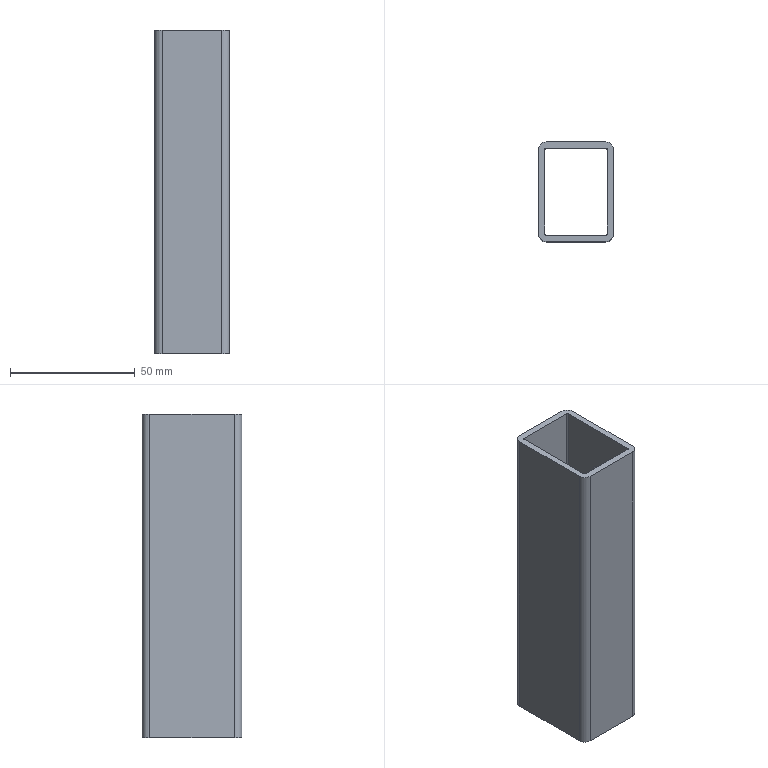Part | SolidWorks | features BaseBody 1 | 1 solid | 22 faces | box 30 x 40 x 130 mm | volume 41175 mm3 | cylinder 12 | plane 10 | commonest cylinder face diameters 1 x4 5 x4 6 x4
STEP:
#1=CARTESIAN_POINT('',(12.5,0.,47.5));
#2=VERTEX_POINT('',#1);
#3=CARTESIAN_POINT('',(15.,0.,47.5));
#4=VERTEX_POINT('',#3);
#5=CARTESIAN_POINT('',(15.,0.,47.5));
#6=DIRECTION('',(1.,0.,0.));
#7=VECTOR('',#6,1000.);
#8=LINE('',#5,#7);
#9=EDGE_CURVE('',#2,#4,#8,.T.);
#10=ORIENTED_EDGE('',*,*,#9,.F.);
#11=CARTESIAN_POINT('',(12.5,0.,42.5));
#12=VERTEX_POINT('',#11);
#13=CARTESIAN_POINT('',(12.5,0.,45.));
#14=DIRECTION('',(-1.,0.,0.));
#15=DIRECTION('',(0.,-1.,0.));
#16=AXIS2_PLACEMENT_3D('',#13,#14,#15);
#17=CIRCLE('',#16,2.5);
#18=EDGE_CURVE('',#2,#12,#17,.T.);
#19=ORIENTED_EDGE('',*,*,#18,.T.);
#20=CARTESIAN_POINT('',(15.,0.,42.5));
#21=VERTEX_POINT('',#20);
#22=CARTESIAN_POINT('',(15.,0.,42.5));
#23=DIRECTION('',(1.,0.,0.));
#24=VECTOR('',#23,1000.);
#25=LINE('',#22,#24);
#26=EDGE_CURVE('',#12,#21,#25,.T.);
#27=ORIENTED_EDGE('',*,*,#26,.T.);
#28=CARTESIAN_POINT('',(15.,0.,45.));
#29=DIRECTION('',(1.,0.,0.));
#30=DIRECTION('',(0.,0.,-1.));
#31=AXIS2_PLACEMENT_3D('',#28,#29,#30);
#32=CIRCLE('',#31,2.5);
#33=EDGE_CURVE('',#21,#4,#32,.T.);
#34=ORIENTED_EDGE('',*,*,#33,.T.);
#35=EDGE_LOOP('',(#10,#19,#27,#34));
#36=FACE_OUTER_BOUND('',#35,.T.);
#37=CARTESIAN_POINT('',(15.,0.,45.));
#38=DIRECTION('',(1.,0.,0.));
#39=DIRECTION('',(0.,0.,-1.));
#40=AXIS2_PLACEMENT_3D('',#37,#38,#39);
#41=CYLINDRICAL_SURFACE('',#40,2.5);
#42=ADVANCED_FACE('',(#36),#41,.F.);
#43=CARTESIAN_POINT('',(12.5,0.,-42.5));
#44=VERTEX_POINT('',#43);
#45=CARTESIAN_POINT('',(15.,0.,-42.5));
#46=VERTEX_POINT('',#45);
#47=CARTESIAN_POINT('',(15.,0.,-42.5));
#48=DIRECTION('',(1.,0.,0.));
#49=VECTOR('',#48,1000.);
#50=LINE('',#47,#49);
#51=EDGE_CURVE('',#44,#46,#50,.T.);
#52=ORIENTED_EDGE('',*,*,#51,.F.);
#53=CARTESIAN_POINT('',(12.5,0.,-47.5));
#54=VERTEX_POINT('',#53);
#55=CARTESIAN_POINT('',(12.5,0.,-45.));
#56=DIRECTION('',(-1.,0.,0.));
#57=DIRECTION('',(0.,-1.,0.));
#58=AXIS2_PLACEMENT_3D('',#55,#56,#57);
#59=CIRCLE('',#58,2.5);
#60=EDGE_CURVE('',#44,#54,#59,.T.);
#61=ORIENTED_EDGE('',*,*,#60,.T.);
#62=CARTESIAN_POINT('',(15.,0.,-47.5));
#63=VERTEX_POINT('',#62);
#64=CARTESIAN_POINT('',(15.,0.,-47.5));
#65=DIRECTION('',(1.,0.,0.));
#66=VECTOR('',#65,1000.);
#67=LINE('',#64,#66);
#68=EDGE_CURVE('',#54,#63,#67,.T.);
#69=ORIENTED_EDGE('',*,*,#68,.T.);
#70=CARTESIAN_POINT('',(15.,0.,-45.));
#71=DIRECTION('',(1.,0.,0.));
#72=DIRECTION('',(0.,0.,-1.));
#73=AXIS2_PLACEMENT_3D('',#70,#71,#72);
#74=CIRCLE('',#73,2.5);
#75=EDGE_CURVE('',#63,#46,#74,.T.);
#76=ORIENTED_EDGE('',*,*,#75,.T.);
#77=EDGE_LOOP('',(#52,#61,#69,#76));
#78=FACE_OUTER_BOUND('',#77,.T.);
#79=CARTESIAN_POINT('',(15.,0.,-45.));
#80=DIRECTION('',(1.,0.,0.));
#81=DIRECTION('',(0.,0.,-1.));
#82=AXIS2_PLACEMENT_3D('',#79,#80,#81);
#83=CYLINDRICAL_SURFACE('',#82,2.5);
#84=ADVANCED_FACE('',(#78),#83,.F.);
#85=CARTESIAN_POINT('',(12.,17.5,-65.));
#86=VERTEX_POINT('',#85);
#87=CARTESIAN_POINT('',(-12.,17.5,-65.));
#88=VERTEX_POINT('',#87);
#89=CARTESIAN_POINT('',(-12.,17.5,-65.));
#90=DIRECTION('',(-1.,0.,0.));
#91=VECTOR('',#90,1000.);
#92=LINE('',#89,#91);
#93=EDGE_CURVE('',#86,#88,#92,.T.);
#94=ORIENTED_EDGE('',*,*,#93,.F.);
#95=CARTESIAN_POINT('',(12.,17.5,65.));
#96=VERTEX_POINT('',#95);
#97=CARTESIAN_POINT('',(12.,17.5,65.));
#98=DIRECTION('',(0.,0.,-1.));
#99=VECTOR('',#98,1000.);
#100=LINE('',#97,#99);
#101=EDGE_CURVE('',#96,#86,#100,.T.);
#102=ORIENTED_EDGE('',*,*,#101,.F.);
#103=CARTESIAN_POINT('',(-12.,17.5,65.));
#104=VERTEX_POINT('',#103);
#105=CARTESIAN_POINT('',(-12.,17.5,65.));
#106=DIRECTION('',(-1.,0.,0.));
#107=VECTOR('',#106,1000.);
#108=LINE('',#105,#107);
#109=EDGE_CURVE('',#96,#104,#108,.T.);
#110=ORIENTED_EDGE('',*,*,#109,.T.);
#111=CARTESIAN_POINT('',(-12.,17.5,65.));
#112=DIRECTION('',(0.,0.,-1.));
#113=VECTOR('',#112,1000.);
#114=LINE('',#111,#113);
#115=EDGE_CURVE('',#104,#88,#114,.T.);
#116=ORIENTED_EDGE('',*,*,#115,.T.);
#117=EDGE_LOOP('',(#94,#102,#110,#116));
#118=FACE_OUTER_BOUND('',#117,.T.);
#119=CARTESIAN_POINT('',(-12.,17.5,65.));
#120=DIRECTION('',(0.,-1.,0.));
#121=DIRECTION('',(0.,0.,-1.));
#122=AXIS2_PLACEMENT_3D('',#119,#120,#121);
#123=PLANE('',#122);
#124=ADVANCED_FACE('',(#118),#123,.T.);
#125=CARTESIAN_POINT('',(12.5,17.,-65.));
#126=VERTEX_POINT('',#125);
#127=CARTESIAN_POINT('',(12.,17.,-65.));
#128=DIRECTION('',(0.,0.,1.));
#129=DIRECTION('',(-1.,0.,0.));
#130=AXIS2_PLACEMENT_3D('',#127,#128,#129);
#131=CIRCLE('',#130,0.5);
#132=EDGE_CURVE('',#126,#86,#131,.T.);
#133=ORIENTED_EDGE('',*,*,#132,.F.);
#134=CARTESIAN_POINT('',(12.5,17.,65.));
#135=VERTEX_POINT('',#134);
#136=CARTESIAN_POINT('',(12.5,17.,65.));
#137=DIRECTION('',(0.,0.,-1.));
#138=VECTOR('',#137,1000.);
#139=LINE('',#136,#138);
#140=EDGE_CURVE('',#135,#126,#139,.T.);
#141=ORIENTED_EDGE('',*,*,#140,.F.);
#142=CARTESIAN_POINT('',(12.,17.,65.));
#143=DIRECTION('',(0.,0.,1.));
#144=DIRECTION('',(-1.,0.,0.));
#145=AXIS2_PLACEMENT_3D('',#142,#143,#144);
#146=CIRCLE('',#145,0.5);
#147=EDGE_CURVE('',#135,#96,#146,.T.);
#148=ORIENTED_EDGE('',*,*,#147,.T.);
#149=ORIENTED_EDGE('',*,*,#101,.T.);
#150=EDGE_LOOP('',(#133,#141,#148,#149));
#151=FACE_OUTER_BOUND('',#150,.T.);
#152=CARTESIAN_POINT('',(12.,17.,65.));
#153=DIRECTION('',(0.,0.,-1.));
#154=DIRECTION('',(-1.,0.,0.));
#155=AXIS2_PLACEMENT_3D('',#152,#153,#154);
#156=CYLINDRICAL_SURFACE('',#155,0.5);
#157=ADVANCED_FACE('',(#151),#156,.F.);
#158=CARTESIAN_POINT('',(12.5,0.,-45.));
#159=DIRECTION('',(-1.,0.,0.));
#160=DIRECTION('',(0.,-1.,0.));
#161=AXIS2_PLACEMENT_3D('',#158,#159,#160);
#162=CIRCLE('',#161,2.5);
#163=EDGE_CURVE('',#54,#44,#162,.T.);
#164=ORIENTED_EDGE('',*,*,#163,.F.);
#165=ORIENTED_EDGE('',*,*,#60,.F.);
#166=EDGE_LOOP('',(#164,#165));
#167=FACE_BOUND('',#166,.T.);
#168=CARTESIAN_POINT('',(12.5,0.,45.));
#169=DIRECTION('',(-1.,0.,0.));
#170=DIRECTION('',(0.,-1.,0.));
#171=AXIS2_PLACEMENT_3D('',#168,#169,#170);
#172=CIRCLE('',#171,2.5);
#173=EDGE_CURVE('',#12,#2,#172,.T.);
#174=ORIENTED_EDGE('',*,*,#173,.F.);
#175=ORIENTED_EDGE('',*,*,#18,.F.);
#176=EDGE_LOOP('',(#174,#175));
#177=FACE_BOUND('',#176,.T.);
#178=CARTESIAN_POINT('',(12.5,-17.,-65.));
#179=VERTEX_POINT('',#178);
#180=CARTESIAN_POINT('',(12.5,17.,-65.));
#181=DIRECTION('',(0.,1.,0.));
#182=VECTOR('',#181,1000.);
#183=LINE('',#180,#182);
#184=EDGE_CURVE('',#179,#126,#183,.T.);
#185=ORIENTED_EDGE('',*,*,#184,.F.);
#186=CARTESIAN_POINT('',(12.5,-17.,65.));
#187=VERTEX_POINT('',#186);
#188=CARTESIAN_POINT('',(12.5,-17.,65.));
#189=DIRECTION('',(0.,0.,-1.));
#190=VECTOR('',#189,1000.);
#191=LINE('',#188,#190);
#192=EDGE_CURVE('',#187,#179,#191,.T.);
#193=ORIENTED_EDGE('',*,*,#192,.F.);
#194=CARTESIAN_POINT('',(12.5,17.,65.));
#195=DIRECTION('',(0.,1.,0.));
#196=VECTOR('',#195,1000.);
#197=LINE('',#194,#196);
#198=EDGE_CURVE('',#187,#135,#197,.T.);
#199=ORIENTED_EDGE('',*,*,#198,.T.);
#200=ORIENTED_EDGE('',*,*,#140,.T.);
#201=EDGE_LOOP('',(#185,#193,#199,#200));
#202=FACE_OUTER_BOUND('',#201,.T.);
#203=CARTESIAN_POINT('',(12.5,17.,65.));
#204=DIRECTION('',(-1.,0.,0.));
#205=DIRECTION('',(0.,1.,0.));
#206=AXIS2_PLACEMENT_3D('',#203,#204,#205);
#207=PLANE('',#206);
#208=ADVANCED_FACE('',(#167,#177,#202),#207,.T.);
#209=CARTESIAN_POINT('',(12.,-17.5,-65.));
#210=VERTEX_POINT('',#209);
#211=CARTESIAN_POINT('',(12.,-17.,-65.));
#212=DIRECTION('',(0.,0.,1.));
#213=DIRECTION('',(1.,0.,0.));
#214=AXIS2_PLACEMENT_3D('',#211,#212,#213);
#215=CIRCLE('',#214,0.5);
#216=EDGE_CURVE('',#210,#179,#215,.T.);
#217=ORIENTED_EDGE('',*,*,#216,.F.);
#218=CARTESIAN_POINT('',(12.,-17.5,65.));
#219=VERTEX_POINT('',#218);
#220=CARTESIAN_POINT('',(12.,-17.5,65.));
#221=DIRECTION('',(0.,0.,-1.));
#222=VECTOR('',#221,1000.);
#223=LINE('',#220,#222);
#224=EDGE_CURVE('',#219,#210,#223,.T.);
#225=ORIENTED_EDGE('',*,*,#224,.F.);
#226=CARTESIAN_POINT('',(12.,-17.,65.));
#227=DIRECTION('',(0.,0.,1.));
#228=DIRECTION('',(1.,0.,0.));
#229=AXIS2_PLACEMENT_3D('',#226,#227,#228);
#230=CIRCLE('',#229,0.5);
#231=EDGE_CURVE('',#219,#187,#230,.T.);
#232=ORIENTED_EDGE('',*,*,#231,.T.);
#233=ORIENTED_EDGE('',*,*,#192,.T.);
#234=EDGE_LOOP('',(#217,#225,#232,#233));
#235=FACE_OUTER_BOUND('',#234,.T.);
#236=CARTESIAN_POINT('',(12.,-17.,65.));
#237=DIRECTION('',(0.,0.,-1.));
#238=DIRECTION('',(-1.,0.,0.));
#239=AXIS2_PLACEMENT_3D('',#236,#237,#238);
#240=CYLINDRICAL_SURFACE('',#239,0.5);
#241=ADVANCED_FACE('',(#235),#240,.F.);
#242=CARTESIAN_POINT('',(-12.,-17.5,-65.));
#243=VERTEX_POINT('',#242);
#244=CARTESIAN_POINT('',(-12.,-17.5,-65.));
#245=DIRECTION('',(1.,0.,0.));
#246=VECTOR('',#245,1000.);
#247=LINE('',#244,#246);
#248=EDGE_CURVE('',#243,#210,#247,.T.);
#249=ORIENTED_EDGE('',*,*,#248,.F.);
#250=CARTESIAN_POINT('',(-12.,-17.5,65.));
#251=VERTEX_POINT('',#250);
#252=CARTESIAN_POINT('',(-12.,-17.5,65.));
#253=DIRECTION('',(0.,0.,-1.));
#254=VECTOR('',#253,1000.);
#255=LINE('',#252,#254);
#256=EDGE_CURVE('',#251,#243,#255,.T.);
#257=ORIENTED_EDGE('',*,*,#256,.F.);
#258=CARTESIAN_POINT('',(-12.,-17.5,65.));
#259=DIRECTION('',(1.,0.,0.));
#260=VECTOR('',#259,1000.);
#261=LINE('',#258,#260);
#262=EDGE_CURVE('',#251,#219,#261,.T.);
#263=ORIENTED_EDGE('',*,*,#262,.T.);
#264=ORIENTED_EDGE('',*,*,#224,.T.);
#265=EDGE_LOOP('',(#249,#257,#263,#264));
#266=FACE_OUTER_BOUND('',#265,.T.);
#267=CARTESIAN_POINT('',(-12.,-17.5,65.));
#268=DIRECTION('',(0.,1.,0.));
#269=DIRECTION('',(1.,0.,0.));
#270=AXIS2_PLACEMENT_3D('',#267,#268,#269);
#271=PLANE('',#270);
#272=ADVANCED_FACE('',(#266),#271,.T.);
#273=CARTESIAN_POINT('',(-12.5,-17.,-65.));
#274=VERTEX_POINT('',#273);
#275=CARTESIAN_POINT('',(-12.,-17.,-65.));
#276=DIRECTION('',(0.,0.,1.));
#277=DIRECTION('',(1.,0.,0.));
#278=AXIS2_PLACEMENT_3D('',#275,#276,#277);
#279=CIRCLE('',#278,0.5);
#280=EDGE_CURVE('',#274,#243,#279,.T.);
#281=ORIENTED_EDGE('',*,*,#280,.F.);
#282=CARTESIAN_POINT('',(-12.5,-17.,65.));
#283=VERTEX_POINT('',#282);
#284=CARTESIAN_POINT('',(-12.5,-17.,65.));
#285=DIRECTION('',(0.,0.,-1.));
#286=VECTOR('',#285,1000.);
#287=LINE('',#284,#286);
#288=EDGE_CURVE('',#283,#274,#287,.T.);
#289=ORIENTED_EDGE('',*,*,#288,.F.);
#290=CARTESIAN_POINT('',(-12.,-17.,65.));
#291=DIRECTION('',(0.,0.,1.));
#292=DIRECTION('',(1.,0.,0.));
#293=AXIS2_PLACEMENT_3D('',#290,#291,#292);
#294=CIRCLE('',#293,0.5);
#295=EDGE_CURVE('',#283,#251,#294,.T.);
#296=ORIENTED_EDGE('',*,*,#295,.T.);
#297=ORIENTED_EDGE('',*,*,#256,.T.);
#298=EDGE_LOOP('',(#281,#289,#296,#297));
#299=FACE_OUTER_BOUND('',#298,.T.);
#300=CARTESIAN_POINT('',(-12.,-17.,65.));
#301=DIRECTION('',(0.,0.,-1.));
#302=DIRECTION('',(-1.,0.,0.));
#303=AXIS2_PLACEMENT_3D('',#300,#301,#302);
#304=CYLINDRICAL_SURFACE('',#303,0.5);
#305=ADVANCED_FACE('',(#299),#304,.F.);
#306=CARTESIAN_POINT('',(-12.5,17.,-65.));
#307=VERTEX_POINT('',#306);
#308=CARTESIAN_POINT('',(-12.5,17.,-65.));
#309=DIRECTION('',(0.,-1.,0.));
#310=VECTOR('',#309,1000.);
#311=LINE('',#308,#310);
#312=EDGE_CURVE('',#307,#274,#311,.T.);
#313=ORIENTED_EDGE('',*,*,#312,.F.);
#314=CARTESIAN_POINT('',(-12.5,17.,65.));
#315=VERTEX_POINT('',#314);
#316=CARTESIAN_POINT('',(-12.5,17.,65.));
#317=DIRECTION('',(0.,0.,-1.));
#318=VECTOR('',#317,1000.);
#319=LINE('',#316,#318);
#320=EDGE_CURVE('',#315,#307,#319,.T.);
#321=ORIENTED_EDGE('',*,*,#320,.F.);
#322=CARTESIAN_POINT('',(-12.5,17.,65.));
#323=DIRECTION('',(0.,-1.,0.));
#324=VECTOR('',#323,1000.);
#325=LINE('',#322,#324);
#326=EDGE_CURVE('',#315,#283,#325,.T.);
#327=ORIENTED_EDGE('',*,*,#326,.T.);
#328=ORIENTED_EDGE('',*,*,#288,.T.);
#329=EDGE_LOOP('',(#313,#321,#327,#328));
#330=FACE_OUTER_BOUND('',#329,.T.);
#331=CARTESIAN_POINT('',(-12.5,17.,65.));
#332=DIRECTION('',(1.,0.,0.));
#333=DIRECTION('',(0.,1.,0.));
#334=AXIS2_PLACEMENT_3D('',#331,#332,#333);
#335=PLANE('',#334);
#336=ADVANCED_FACE('',(#330),#335,.T.);
#337=CARTESIAN_POINT('',(-12.,17.,-65.));
#338=DIRECTION('',(0.,0.,1.));
#339=DIRECTION('',(1.,0.,0.));
#340=AXIS2_PLACEMENT_3D('',#337,#338,#339);
#341=CIRCLE('',#340,0.5);
#342=EDGE_CURVE('',#88,#307,#341,.T.);
#343=ORIENTED_EDGE('',*,*,#342,.F.);
#344=ORIENTED_EDGE('',*,*,#115,.F.);
#345=CARTESIAN_POINT('',(-12.,17.,65.));
#346=DIRECTION('',(0.,0.,1.));
#347=DIRECTION('',(1.,0.,0.));
#348=AXIS2_PLACEMENT_3D('',#345,#346,#347);
#349=CIRCLE('',#348,0.5);
#350=EDGE_CURVE('',#104,#315,#349,.T.);
#351=ORIENTED_EDGE('',*,*,#350,.T.);
#352=ORIENTED_EDGE('',*,*,#320,.T.);
#353=EDGE_LOOP('',(#343,#344,#351,#352));
#354=FACE_OUTER_BOUND('',#353,.T.);
#355=CARTESIAN_POINT('',(-12.,17.,65.));
#356=DIRECTION('',(0.,0.,-1.));
#357=DIRECTION('',(-1.,0.,0.));
#358=AXIS2_PLACEMENT_3D('',#355,#356,#357);
#359=CYLINDRICAL_SURFACE('',#358,0.5);
#360=ADVANCED_FACE('',(#354),#359,.F.);
#361=CARTESIAN_POINT('',(-15.,17.,-65.));
#362=VERTEX_POINT('',#361);
#363=CARTESIAN_POINT('',(-15.,-17.,-65.));
#364=VERTEX_POINT('',#363);
#365=CARTESIAN_POINT('',(-15.,17.,-65.));
#366=DIRECTION('',(0.,-1.,0.));
#367=VECTOR('',#366,1000.);
#368=LINE('',#365,#367);
#369=EDGE_CURVE('',#362,#364,#368,.T.);
#370=ORIENTED_EDGE('',*,*,#369,.T.);
#371=CARTESIAN_POINT('',(-15.,-17.,65.));
#372=VERTEX_POINT('',#371);
#373=CARTESIAN_POINT('',(-15.,-17.,65.));
#374=DIRECTION('',(0.,0.,-1.));
#375=VECTOR('',#374,1000.);
#376=LINE('',#373,#375);
#377=EDGE_CURVE('',#372,#364,#376,.T.);
#378=ORIENTED_EDGE('',*,*,#377,.F.);
#379=CARTESIAN_POINT('',(-15.,17.,65.));
#380=VERTEX_POINT('',#379);
#381=CARTESIAN_POINT('',(-15.,17.,65.));
#382=DIRECTION('',(0.,-1.,0.));
#383=VECTOR('',#382,1000.);
#384=LINE('',#381,#383);
#385=EDGE_CURVE('',#380,#372,#384,.T.);
#386=ORIENTED_EDGE('',*,*,#385,.F.);
#387=CARTESIAN_POINT('',(-15.,17.,65.));
#388=DIRECTION('',(0.,0.,-1.));
#389=VECTOR('',#388,1000.);
#390=LINE('',#387,#389);
#391=EDGE_CURVE('',#380,#362,#390,.T.);
#392=ORIENTED_EDGE('',*,*,#391,.T.);
#393=EDGE_LOOP('',(#370,#378,#386,#392));
#394=FACE_OUTER_BOUND('',#393,.T.);
#395=CARTESIAN_POINT('',(-15.,17.,65.));
#396=DIRECTION('',(1.,0.,0.));
#397=DIRECTION('',(0.,1.,0.));
#398=AXIS2_PLACEMENT_3D('',#395,#396,#397);
#399=PLANE('',#398);
#400=ADVANCED_FACE('',(#394),#399,.F.);
#401=CARTESIAN_POINT('',(-12.,20.,-65.));
#402=VERTEX_POINT('',#401);
#403=CARTESIAN_POINT('',(-12.,17.,-65.));
#404=DIRECTION('',(0.,0.,1.));
#405=DIRECTION('',(1.,0.,0.));
#406=AXIS2_PLACEMENT_3D('',#403,#404,#405);
#407=CIRCLE('',#406,3.);
#408=EDGE_CURVE('',#402,#362,#407,.T.);
#409=ORIENTED_EDGE('',*,*,#408,.T.);
#410=ORIENTED_EDGE('',*,*,#391,.F.);
#411=CARTESIAN_POINT('',(-12.,20.,65.));
#412=VERTEX_POINT('',#411);
#413=CARTESIAN_POINT('',(-12.,17.,65.));
#414=DIRECTION('',(0.,0.,1.));
#415=DIRECTION('',(1.,0.,0.));
#416=AXIS2_PLACEMENT_3D('',#413,#414,#415);
#417=CIRCLE('',#416,3.);
#418=EDGE_CURVE('',#412,#380,#417,.T.);
#419=ORIENTED_EDGE('',*,*,#418,.F.);
#420=CARTESIAN_POINT('',(-12.,20.,65.));
#421=DIRECTION('',(0.,0.,-1.));
#422=VECTOR('',#421,1000.);
#423=LINE('',#420,#422);
#424=EDGE_CURVE('',#412,#402,#423,.T.);
#425=ORIENTED_EDGE('',*,*,#424,.T.);
#426=EDGE_LOOP('',(#409,#410,#419,#425));
#427=FACE_OUTER_BOUND('',#426,.T.);
#428=CARTESIAN_POINT('',(-12.,17.,65.));
#429=DIRECTION('',(0.,0.,-1.));
#430=DIRECTION('',(-1.,0.,0.));
#431=AXIS2_PLACEMENT_3D('',#428,#429,#430);
#432=CYLINDRICAL_SURFACE('',#431,3.);
#433=ADVANCED_FACE('',(#427),#432,.T.);
#434=CARTESIAN_POINT('',(12.,20.,-65.));
#435=VERTEX_POINT('',#434);
#436=CARTESIAN_POINT('',(-12.,20.,-65.));
#437=DIRECTION('',(-1.,0.,0.));
#438=VECTOR('',#437,1000.);
#439=LINE('',#436,#438);
#440=EDGE_CURVE('',#435,#402,#439,.T.);
#441=ORIENTED_EDGE('',*,*,#440,.T.);
#442=ORIENTED_EDGE('',*,*,#424,.F.);
#443=CARTESIAN_POINT('',(12.,20.,65.));
#444=VERTEX_POINT('',#443);
#445=CARTESIAN_POINT('',(-12.,20.,65.));
#446=DIRECTION('',(-1.,0.,0.));
#447=VECTOR('',#446,1000.);
#448=LINE('',#445,#447);
#449=EDGE_CURVE('',#444,#412,#448,.T.);
#450=ORIENTED_EDGE('',*,*,#449,.F.);
#451=CARTESIAN_POINT('',(12.,20.,65.));
#452=DIRECTION('',(0.,0.,-1.));
#453=VECTOR('',#452,1000.);
#454=LINE('',#451,#453);
#455=EDGE_CURVE('',#444,#435,#454,.T.);
#456=ORIENTED_EDGE('',*,*,#455,.T.);
#457=EDGE_LOOP('',(#441,#442,#450,#456));
#458=FACE_OUTER_BOUND('',#457,.T.);
#459=CARTESIAN_POINT('',(-12.,20.,65.));
#460=DIRECTION('',(0.,-1.,0.));
#461=DIRECTION('',(0.,0.,-1.));
#462=AXIS2_PLACEMENT_3D('',#459,#460,#461);
#463=PLANE('',#462);
#464=ADVANCED_FACE('',(#458),#463,.F.);
#465=CARTESIAN_POINT('',(15.,17.,-65.));
#466=VERTEX_POINT('',#465);
#467=CARTESIAN_POINT('',(12.,17.,-65.));
#468=DIRECTION('',(0.,0.,1.));
#469=DIRECTION('',(-1.,0.,0.));
#470=AXIS2_PLACEMENT_3D('',#467,#468,#469);
#471=CIRCLE('',#470,3.);
#472=EDGE_CURVE('',#466,#435,#471,.T.);
#473=ORIENTED_EDGE('',*,*,#472,.T.);
#474=ORIENTED_EDGE('',*,*,#455,.F.);
#475=CARTESIAN_POINT('',(15.,17.,65.));
#476=VERTEX_POINT('',#475);
#477=CARTESIAN_POINT('',(12.,17.,65.));
#478=DIRECTION('',(0.,0.,1.));
#479=DIRECTION('',(-1.,0.,0.));
#480=AXIS2_PLACEMENT_3D('',#477,#478,#479);
#481=CIRCLE('',#480,3.);
#482=EDGE_CURVE('',#476,#444,#481,.T.);
#483=ORIENTED_EDGE('',*,*,#482,.F.);
#484=CARTESIAN_POINT('',(15.,17.,65.));
#485=DIRECTION('',(0.,0.,-1.));
#486=VECTOR('',#485,1000.);
#487=LINE('',#484,#486);
#488=EDGE_CURVE('',#476,#466,#487,.T.);
#489=ORIENTED_EDGE('',*,*,#488,.T.);
#490=EDGE_LOOP('',(#473,#474,#483,#489));
#491=FACE_OUTER_BOUND('',#490,.T.);
#492=CARTESIAN_POINT('',(12.,17.,65.));
#493=DIRECTION('',(0.,0.,-1.));
#494=DIRECTION('',(-1.,0.,0.));
#495=AXIS2_PLACEMENT_3D('',#492,#493,#494);
#496=CYLINDRICAL_SURFACE('',#495,3.);
#497=ADVANCED_FACE('',(#491),#496,.T.);
#498=CARTESIAN_POINT('',(12.,-20.,-65.));
#499=VERTEX_POINT('',#498);
#500=CARTESIAN_POINT('',(15.,-17.,-65.));
#501=VERTEX_POINT('',#500);
#502=CARTESIAN_POINT('',(12.,-17.,-65.));
#503=DIRECTION('',(0.,0.,1.));
#504=DIRECTION('',(1.,0.,0.));
#505=AXIS2_PLACEMENT_3D('',#502,#503,#504);
#506=CIRCLE('',#505,3.);
#507=EDGE_CURVE('',#499,#501,#506,.T.);
#508=ORIENTED_EDGE('',*,*,#507,.T.);
#509=CARTESIAN_POINT('',(15.,-17.,65.));
#510=VERTEX_POINT('',#509);
#511=CARTESIAN_POINT('',(15.,-17.,65.));
#512=DIRECTION('',(0.,0.,-1.));
#513=VECTOR('',#512,1000.);
#514=LINE('',#511,#513);
#515=EDGE_CURVE('',#510,#501,#514,.T.);
#516=ORIENTED_EDGE('',*,*,#515,.F.);
#517=CARTESIAN_POINT('',(12.,-20.,65.));
#518=VERTEX_POINT('',#517);
#519=CARTESIAN_POINT('',(12.,-17.,65.));
#520=DIRECTION('',(0.,0.,1.));
#521=DIRECTION('',(1.,0.,0.));
#522=AXIS2_PLACEMENT_3D('',#519,#520,#521);
#523=CIRCLE('',#522,3.);
#524=EDGE_CURVE('',#518,#510,#523,.T.);
#525=ORIENTED_EDGE('',*,*,#524,.F.);
#526=CARTESIAN_POINT('',(12.,-20.,65.));
#527=DIRECTION('',(0.,0.,-1.));
#528=VECTOR('',#527,1000.);
#529=LINE('',#526,#528);
#530=EDGE_CURVE('',#518,#499,#529,.T.);
#531=ORIENTED_EDGE('',*,*,#530,.T.);
#532=EDGE_LOOP('',(#508,#516,#525,#531));
#533=FACE_OUTER_BOUND('',#532,.T.);
#534=CARTESIAN_POINT('',(12.,-17.,65.));
#535=DIRECTION('',(0.,0.,-1.));
#536=DIRECTION('',(-1.,0.,0.));
#537=AXIS2_PLACEMENT_3D('',#534,#535,#536);
#538=CYLINDRICAL_SURFACE('',#537,3.);
#539=ADVANCED_FACE('',(#533),#538,.T.);
#540=CARTESIAN_POINT('',(-12.,-20.,-65.));
#541=VERTEX_POINT('',#540);
#542=CARTESIAN_POINT('',(-12.,-20.,-65.));
#543=DIRECTION('',(1.,0.,0.));
#544=VECTOR('',#543,1000.);
#545=LINE('',#542,#544);
#546=EDGE_CURVE('',#541,#499,#545,.T.);
#547=ORIENTED_EDGE('',*,*,#546,.T.);
#548=ORIENTED_EDGE('',*,*,#530,.F.);
#549=CARTESIAN_POINT('',(-12.,-20.,65.));
#550=VERTEX_POINT('',#549);
#551=CARTESIAN_POINT('',(-12.,-20.,65.));
#552=DIRECTION('',(1.,0.,0.));
#553=VECTOR('',#552,1000.);
#554=LINE('',#551,#553);
#555=EDGE_CURVE('',#550,#518,#554,.T.);
#556=ORIENTED_EDGE('',*,*,#555,.F.);
#557=CARTESIAN_POINT('',(-12.,-20.,65.));
#558=DIRECTION('',(0.,0.,-1.));
#559=VECTOR('',#558,1000.);
#560=LINE('',#557,#559);
#561=EDGE_CURVE('',#550,#541,#560,.T.);
#562=ORIENTED_EDGE('',*,*,#561,.T.);
#563=EDGE_LOOP('',(#547,#548,#556,#562));
#564=FACE_OUTER_BOUND('',#563,.T.);
#565=CARTESIAN_POINT('',(-12.,-20.,65.));
#566=DIRECTION('',(0.,1.,0.));
#567=DIRECTION('',(1.,0.,0.));
#568=AXIS2_PLACEMENT_3D('',#565,#566,#567);
#569=PLANE('',#568);
#570=ADVANCED_FACE('',(#564),#569,.F.);
#571=CARTESIAN_POINT('',(-12.,-17.,-65.));
#572=DIRECTION('',(0.,0.,1.));
#573=DIRECTION('',(1.,0.,0.));
#574=AXIS2_PLACEMENT_3D('',#571,#572,#573);
#575=CIRCLE('',#574,3.);
#576=EDGE_CURVE('',#364,#541,#575,.T.);
#577=ORIENTED_EDGE('',*,*,#576,.T.);
#578=ORIENTED_EDGE('',*,*,#561,.F.);
#579=CARTESIAN_POINT('',(-12.,-17.,65.));
#580=DIRECTION('',(0.,0.,1.));
#581=DIRECTION('',(1.,0.,0.));
#582=AXIS2_PLACEMENT_3D('',#579,#580,#581);
#583=CIRCLE('',#582,3.);
#584=EDGE_CURVE('',#372,#550,#583,.T.);
#585=ORIENTED_EDGE('',*,*,#584,.F.);
#586=ORIENTED_EDGE('',*,*,#377,.T.);
#587=EDGE_LOOP('',(#577,#578,#585,#586));
#588=FACE_OUTER_BOUND('',#587,.T.);
#589=CARTESIAN_POINT('',(-12.,-17.,65.));
#590=DIRECTION('',(0.,0.,-1.));
#591=DIRECTION('',(-1.,0.,0.));
#592=AXIS2_PLACEMENT_3D('',#589,#590,#591);
#593=CYLINDRICAL_SURFACE('',#592,3.);
#594=ADVANCED_FACE('',(#588),#593,.T.);
#595=ORIENTED_EDGE('',*,*,#342,.T.);
#596=ORIENTED_EDGE('',*,*,#312,.T.);
#597=ORIENTED_EDGE('',*,*,#280,.T.);
#598=ORIENTED_EDGE('',*,*,#248,.T.);
#599=ORIENTED_EDGE('',*,*,#216,.T.);
#600=ORIENTED_EDGE('',*,*,#184,.T.);
#601=ORIENTED_EDGE('',*,*,#132,.T.);
#602=ORIENTED_EDGE('',*,*,#93,.T.);
#603=EDGE_LOOP('',(#595,#596,#597,#598,#599,#600,#601,#602));
#604=FACE_BOUND('',#603,.T.);
#605=ORIENTED_EDGE('',*,*,#576,.F.);
#606=ORIENTED_EDGE('',*,*,#369,.F.);
#607=ORIENTED_EDGE('',*,*,#408,.F.);
#608=ORIENTED_EDGE('',*,*,#440,.F.);
#609=ORIENTED_EDGE('',*,*,#472,.F.);
#610=CARTESIAN_POINT('',(15.,17.,-65.));
#611=DIRECTION('',(0.,1.,0.));
#612=VECTOR('',#611,1000.);
#613=LINE('',#610,#612);
#614=EDGE_CURVE('',#501,#466,#613,.T.);
#615=ORIENTED_EDGE('',*,*,#614,.F.);
#616=ORIENTED_EDGE('',*,*,#507,.F.);
#617=ORIENTED_EDGE('',*,*,#546,.F.);
#618=EDGE_LOOP('',(#605,#606,#607,#608,#609,#615,#616,#617));
#619=FACE_OUTER_BOUND('',#618,.T.);
#620=CARTESIAN_POINT('',(-12.,-17.,-65.));
#621=DIRECTION('',(0.,0.,1.));
#622=DIRECTION('',(1.,0.,0.));
#623=AXIS2_PLACEMENT_3D('',#620,#621,#622);
#624=PLANE('',#623);
#625=ADVANCED_FACE('',(#604,#619),#624,.F.);
#626=ORIENTED_EDGE('',*,*,#326,.F.);
#627=ORIENTED_EDGE('',*,*,#350,.F.);
#628=ORIENTED_EDGE('',*,*,#109,.F.);
#629=ORIENTED_EDGE('',*,*,#147,.F.);
#630=ORIENTED_EDGE('',*,*,#198,.F.);
#631=ORIENTED_EDGE('',*,*,#231,.F.);
#632=ORIENTED_EDGE('',*,*,#262,.F.);
#633=ORIENTED_EDGE('',*,*,#295,.F.);
#634=EDGE_LOOP('',(#626,#627,#628,#629,#630,#631,#632,#633));
#635=FACE_BOUND('',#634,.T.);
#636=ORIENTED_EDGE('',*,*,#584,.T.);
#637=ORIENTED_EDGE('',*,*,#555,.T.);
#638=ORIENTED_EDGE('',*,*,#524,.T.);
#639=CARTESIAN_POINT('',(15.,17.,65.));
#640=DIRECTION('',(0.,1.,0.));
#641=VECTOR('',#640,1000.);
#642=LINE('',#639,#641);
#643=EDGE_CURVE('',#510,#476,#642,.T.);
#644=ORIENTED_EDGE('',*,*,#643,.T.);
#645=ORIENTED_EDGE('',*,*,#482,.T.);
#646=ORIENTED_EDGE('',*,*,#449,.T.);
#647=ORIENTED_EDGE('',*,*,#418,.T.);
#648=ORIENTED_EDGE('',*,*,#385,.T.);
#649=EDGE_LOOP('',(#636,#637,#638,#644,#645,#646,#647,#648));
#650=FACE_OUTER_BOUND('',#649,.T.);
#651=CARTESIAN_POINT('',(-12.,-17.,65.));
#652=DIRECTION('',(0.,0.,1.));
#653=DIRECTION('',(1.,0.,0.));
#654=AXIS2_PLACEMENT_3D('',#651,#652,#653);
#655=PLANE('',#654);
#656=ADVANCED_FACE('',(#635,#650),#655,.T.);
#657=ORIENTED_EDGE('',*,*,#33,.F.);
#658=CARTESIAN_POINT('',(15.,0.,45.));
#659=DIRECTION('',(1.,0.,0.));
#660=DIRECTION('',(0.,0.,-1.));
#661=AXIS2_PLACEMENT_3D('',#658,#659,#660);
#662=CIRCLE('',#661,2.5);
#663=EDGE_CURVE('',#4,#21,#662,.T.);
#664=ORIENTED_EDGE('',*,*,#663,.F.);
#665=EDGE_LOOP('',(#657,#664));
#666=FACE_BOUND('',#665,.T.);
#667=ORIENTED_EDGE('',*,*,#75,.F.);
#668=CARTESIAN_POINT('',(15.,0.,-45.));
#669=DIRECTION('',(1.,0.,0.));
#670=DIRECTION('',(0.,0.,-1.));
#671=AXIS2_PLACEMENT_3D('',#668,#669,#670);
#672=CIRCLE('',#671,2.5);
#673=EDGE_CURVE('',#46,#63,#672,.T.);
#674=ORIENTED_EDGE('',*,*,#673,.F.);
#675=EDGE_LOOP('',(#667,#674));
#676=FACE_BOUND('',#675,.T.);
#677=ORIENTED_EDGE('',*,*,#614,.T.);
#678=ORIENTED_EDGE('',*,*,#488,.F.);
#679=ORIENTED_EDGE('',*,*,#643,.F.);
#680=ORIENTED_EDGE('',*,*,#515,.T.);
#681=EDGE_LOOP('',(#677,#678,#679,#680));
#682=FACE_OUTER_BOUND('',#681,.T.);
#683=CARTESIAN_POINT('',(15.,17.,65.));
#684=DIRECTION('',(-1.,0.,0.));
#685=DIRECTION('',(0.,1.,0.));
#686=AXIS2_PLACEMENT_3D('',#683,#684,#685);
#687=PLANE('',#686);
#688=ADVANCED_FACE('',(#666,#676,#682),#687,.F.);
#689=ORIENTED_EDGE('',*,*,#163,.T.);
#690=ORIENTED_EDGE('',*,*,#51,.T.);
#691=ORIENTED_EDGE('',*,*,#673,.T.);
#692=ORIENTED_EDGE('',*,*,#68,.F.);
#693=EDGE_LOOP('',(#689,#690,#691,#692));
#694=FACE_OUTER_BOUND('',#693,.T.);
#695=CARTESIAN_POINT('',(15.,0.,-45.));
#696=DIRECTION('',(1.,0.,0.));
#697=DIRECTION('',(0.,0.,-1.));
#698=AXIS2_PLACEMENT_3D('',#695,#696,#697);
#699=CYLINDRICAL_SURFACE('',#698,2.5);
#700=ADVANCED_FACE('',(#694),#699,.F.);
#701=ORIENTED_EDGE('',*,*,#173,.T.);
#702=ORIENTED_EDGE('',*,*,#9,.T.);
#703=ORIENTED_EDGE('',*,*,#663,.T.);
#704=ORIENTED_EDGE('',*,*,#26,.F.);
#705=EDGE_LOOP('',(#701,#702,#703,#704));
#706=FACE_OUTER_BOUND('',#705,.T.);
#707=CARTESIAN_POINT('',(15.,0.,45.));
#708=DIRECTION('',(1.,0.,0.));
#709=DIRECTION('',(0.,0.,-1.));
#710=AXIS2_PLACEMENT_3D('',#707,#708,#709);
#711=CYLINDRICAL_SURFACE('',#710,2.5);
#712=ADVANCED_FACE('',(#706),#711,.F.);
#713=CLOSED_SHELL('',(#42,#84,#124,#157,#208,#241,#272,#305,#336,#360,#400,#433,#464,#497,#539,#570,#594,#625,#656,#688,#700,#712));
#714=MANIFOLD_SOLID_BREP('',#713);
#715=CARTESIAN_POINT('',(0.,0.,0.));
#716=DIRECTION('',(0.,0.,1.));
#717=DIRECTION('',(1.,0.,0.));
#718=AXIS2_PLACEMENT_3D('',#715,#716,#717);
#719=(LENGTH_UNIT()NAMED_UNIT(*)SI_UNIT(.MILLI.,.METRE.));
#720=UNCERTAINTY_MEASURE_WITH_UNIT(LENGTH_MEASURE(0.00001),#719,'','');
#721=(NAMED_UNIT(*)PLANE_ANGLE_UNIT()SI_UNIT($,.RADIAN.));
#722=(NAMED_UNIT(*)SI_UNIT($,.STERADIAN.)SOLID_ANGLE_UNIT());
#723=(GEOMETRIC_REPRESENTATION_CONTEXT(3)GLOBAL_UNCERTAINTY_ASSIGNED_CONTEXT((#720))GLOBAL_UNIT_ASSIGNED_CONTEXT((#719,#721,#722))REPRESENTATION_CONTEXT('',''));
#724=ADVANCED_BREP_SHAPE_REPRESENTATION('',(#714,#718),#723);